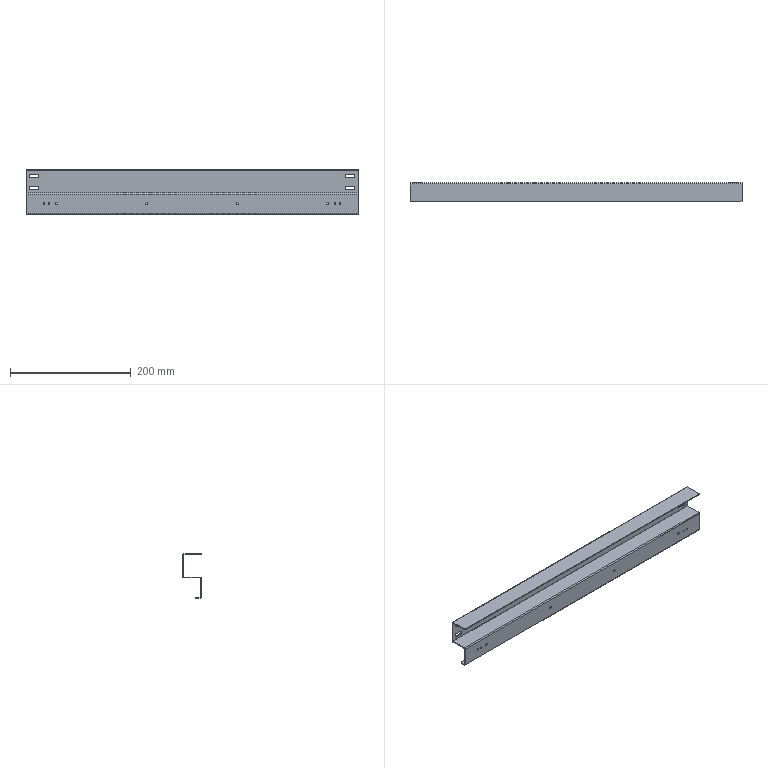Part | STEP file | 1 solid | 74 faces | box 550 x 30 x 73.5 mm | volume 112714 mm3 | plane 38 | cylinder 36 | commonest cylinder face diameters 2.5 x8 3.3 x8 6 x8 0.4 x4 3.4 x4 4 x4